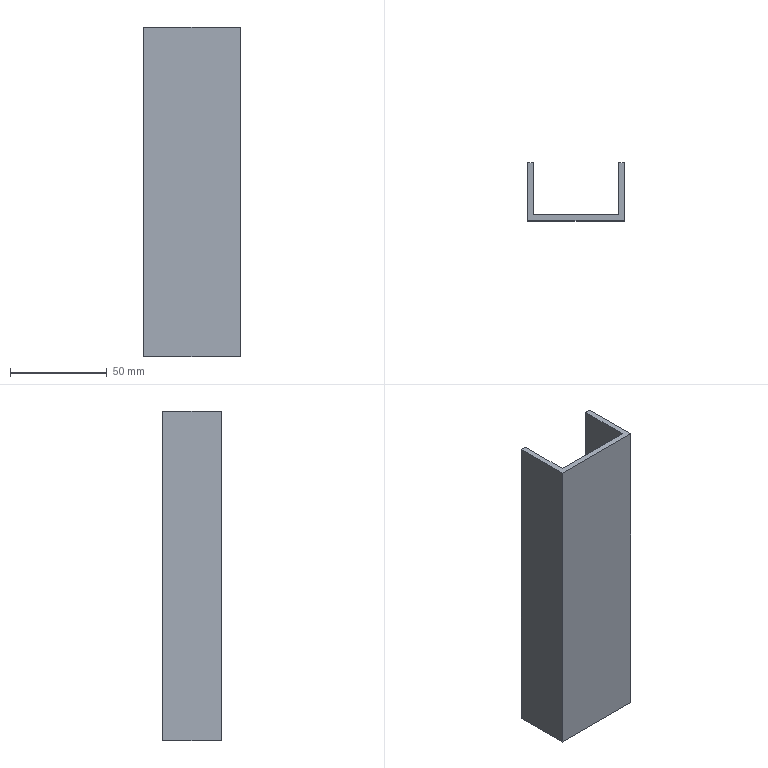Part | SolidWorks | features Extrusion 1, ICE 1 | 1 solid | 10 faces | box 50 x 30 x 170 mm | volume 53040 mm3 | plane 10
STEP:
#1=CARTESIAN_POINT('',(0.,0.,170.));
#2=VERTEX_POINT('',#1);
#3=CARTESIAN_POINT('',(50.,0.,170.));
#4=VERTEX_POINT('',#3);
#5=CARTESIAN_POINT('',(0.,0.,170.));
#6=DIRECTION('',(1.,0.,0.));
#7=VECTOR('',#6,1000.);
#8=LINE('',#5,#7);
#9=EDGE_CURVE('',#2,#4,#8,.T.);
#10=ORIENTED_EDGE('',*,*,#9,.F.);
#11=CARTESIAN_POINT('',(0.,0.,0.));
#12=VERTEX_POINT('',#11);
#13=CARTESIAN_POINT('',(0.,0.,340.));
#14=DIRECTION('',(0.,0.,-1.));
#15=VECTOR('',#14,1000.);
#16=LINE('',#13,#15);
#17=EDGE_CURVE('',#2,#12,#16,.T.);
#18=ORIENTED_EDGE('',*,*,#17,.T.);
#19=CARTESIAN_POINT('',(50.,0.,0.));
#20=VERTEX_POINT('',#19);
#21=CARTESIAN_POINT('',(0.,0.,0.));
#22=DIRECTION('',(1.,0.,0.));
#23=VECTOR('',#22,1000.);
#24=LINE('',#21,#23);
#25=EDGE_CURVE('',#12,#20,#24,.T.);
#26=ORIENTED_EDGE('',*,*,#25,.T.);
#27=CARTESIAN_POINT('',(50.,0.,340.));
#28=DIRECTION('',(0.,0.,-1.));
#29=VECTOR('',#28,1000.);
#30=LINE('',#27,#29);
#31=EDGE_CURVE('',#4,#20,#30,.T.);
#32=ORIENTED_EDGE('',*,*,#31,.F.);
#33=EDGE_LOOP('',(#10,#18,#26,#32));
#34=FACE_OUTER_BOUND('',#33,.T.);
#35=CARTESIAN_POINT('',(0.,0.,340.));
#36=DIRECTION('',(0.,1.,0.));
#37=DIRECTION('',(0.,0.,1.));
#38=AXIS2_PLACEMENT_3D('',#35,#36,#37);
#39=PLANE('',#38);
#40=ADVANCED_FACE('',(#34),#39,.F.);
#41=CARTESIAN_POINT('',(50.,30.,170.));
#42=VERTEX_POINT('',#41);
#43=CARTESIAN_POINT('',(50.,0.,170.));
#44=DIRECTION('',(0.,1.,0.));
#45=VECTOR('',#44,1000.);
#46=LINE('',#43,#45);
#47=EDGE_CURVE('',#4,#42,#46,.T.);
#48=ORIENTED_EDGE('',*,*,#47,.F.);
#49=ORIENTED_EDGE('',*,*,#31,.T.);
#50=CARTESIAN_POINT('',(50.,30.,0.));
#51=VERTEX_POINT('',#50);
#52=CARTESIAN_POINT('',(50.,0.,0.));
#53=DIRECTION('',(0.,1.,0.));
#54=VECTOR('',#53,1000.);
#55=LINE('',#52,#54);
#56=EDGE_CURVE('',#20,#51,#55,.T.);
#57=ORIENTED_EDGE('',*,*,#56,.T.);
#58=CARTESIAN_POINT('',(50.,30.,340.));
#59=DIRECTION('',(0.,0.,-1.));
#60=VECTOR('',#59,1000.);
#61=LINE('',#58,#60);
#62=EDGE_CURVE('',#42,#51,#61,.T.);
#63=ORIENTED_EDGE('',*,*,#62,.F.);
#64=EDGE_LOOP('',(#48,#49,#57,#63));
#65=FACE_OUTER_BOUND('',#64,.T.);
#66=CARTESIAN_POINT('',(50.,0.,340.));
#67=DIRECTION('',(-1.,0.,0.));
#68=DIRECTION('',(0.,0.,1.));
#69=AXIS2_PLACEMENT_3D('',#66,#67,#68);
#70=PLANE('',#69);
#71=ADVANCED_FACE('',(#65),#70,.F.);
#72=CARTESIAN_POINT('',(47.,30.,170.));
#73=VERTEX_POINT('',#72);
#74=CARTESIAN_POINT('',(50.,30.,170.));
#75=DIRECTION('',(-1.,0.,0.));
#76=VECTOR('',#75,1000.);
#77=LINE('',#74,#76);
#78=EDGE_CURVE('',#42,#73,#77,.T.);
#79=ORIENTED_EDGE('',*,*,#78,.F.);
#80=ORIENTED_EDGE('',*,*,#62,.T.);
#81=CARTESIAN_POINT('',(47.,30.,0.));
#82=VERTEX_POINT('',#81);
#83=CARTESIAN_POINT('',(47.,30.,0.));
#84=DIRECTION('',(-1.,0.,0.));
#85=VECTOR('',#84,1000.);
#86=LINE('',#83,#85);
#87=EDGE_CURVE('',#51,#82,#86,.T.);
#88=ORIENTED_EDGE('',*,*,#87,.T.);
#89=CARTESIAN_POINT('',(47.,30.,340.));
#90=DIRECTION('',(0.,0.,-1.));
#91=VECTOR('',#90,1000.);
#92=LINE('',#89,#91);
#93=EDGE_CURVE('',#73,#82,#92,.T.);
#94=ORIENTED_EDGE('',*,*,#93,.F.);
#95=EDGE_LOOP('',(#79,#80,#88,#94));
#96=FACE_OUTER_BOUND('',#95,.T.);
#97=CARTESIAN_POINT('',(47.,30.,340.));
#98=DIRECTION('',(0.,-1.,0.));
#99=DIRECTION('',(0.,0.,-1.));
#100=AXIS2_PLACEMENT_3D('',#97,#98,#99);
#101=PLANE('',#100);
#102=ADVANCED_FACE('',(#96),#101,.F.);
#103=CARTESIAN_POINT('',(47.,3.,170.));
#104=VERTEX_POINT('',#103);
#105=CARTESIAN_POINT('',(47.,30.,170.));
#106=DIRECTION('',(0.,-1.,0.));
#107=VECTOR('',#106,1000.);
#108=LINE('',#105,#107);
#109=EDGE_CURVE('',#73,#104,#108,.T.);
#110=ORIENTED_EDGE('',*,*,#109,.F.);
#111=ORIENTED_EDGE('',*,*,#93,.T.);
#112=CARTESIAN_POINT('',(47.,3.,0.));
#113=VERTEX_POINT('',#112);
#114=CARTESIAN_POINT('',(47.,3.,0.));
#115=DIRECTION('',(0.,-1.,0.));
#116=VECTOR('',#115,1000.);
#117=LINE('',#114,#116);
#118=EDGE_CURVE('',#82,#113,#117,.T.);
#119=ORIENTED_EDGE('',*,*,#118,.T.);
#120=CARTESIAN_POINT('',(47.,3.,340.));
#121=DIRECTION('',(0.,0.,-1.));
#122=VECTOR('',#121,1000.);
#123=LINE('',#120,#122);
#124=EDGE_CURVE('',#104,#113,#123,.T.);
#125=ORIENTED_EDGE('',*,*,#124,.F.);
#126=EDGE_LOOP('',(#110,#111,#119,#125));
#127=FACE_OUTER_BOUND('',#126,.T.);
#128=CARTESIAN_POINT('',(47.,3.,340.));
#129=DIRECTION('',(1.,0.,0.));
#130=DIRECTION('',(0.,0.,-1.));
#131=AXIS2_PLACEMENT_3D('',#128,#129,#130);
#132=PLANE('',#131);
#133=ADVANCED_FACE('',(#127),#132,.F.);
#134=CARTESIAN_POINT('',(3.,3.,170.));
#135=VERTEX_POINT('',#134);
#136=CARTESIAN_POINT('',(47.,3.,170.));
#137=DIRECTION('',(-1.,0.,0.));
#138=VECTOR('',#137,1000.);
#139=LINE('',#136,#138);
#140=EDGE_CURVE('',#104,#135,#139,.T.);
#141=ORIENTED_EDGE('',*,*,#140,.F.);
#142=ORIENTED_EDGE('',*,*,#124,.T.);
#143=CARTESIAN_POINT('',(3.,3.,0.));
#144=VERTEX_POINT('',#143);
#145=CARTESIAN_POINT('',(3.,3.,0.));
#146=DIRECTION('',(-1.,0.,0.));
#147=VECTOR('',#146,1000.);
#148=LINE('',#145,#147);
#149=EDGE_CURVE('',#113,#144,#148,.T.);
#150=ORIENTED_EDGE('',*,*,#149,.T.);
#151=CARTESIAN_POINT('',(3.,3.,340.));
#152=DIRECTION('',(0.,0.,-1.));
#153=VECTOR('',#152,1000.);
#154=LINE('',#151,#153);
#155=EDGE_CURVE('',#135,#144,#154,.T.);
#156=ORIENTED_EDGE('',*,*,#155,.F.);
#157=EDGE_LOOP('',(#141,#142,#150,#156));
#158=FACE_OUTER_BOUND('',#157,.T.);
#159=CARTESIAN_POINT('',(3.,3.,340.));
#160=DIRECTION('',(0.,-1.,0.));
#161=DIRECTION('',(0.,0.,-1.));
#162=AXIS2_PLACEMENT_3D('',#159,#160,#161);
#163=PLANE('',#162);
#164=ADVANCED_FACE('',(#158),#163,.F.);
#165=CARTESIAN_POINT('',(3.,30.,170.));
#166=VERTEX_POINT('',#165);
#167=CARTESIAN_POINT('',(3.,3.,170.));
#168=DIRECTION('',(0.,1.,0.));
#169=VECTOR('',#168,1000.);
#170=LINE('',#167,#169);
#171=EDGE_CURVE('',#135,#166,#170,.T.);
#172=ORIENTED_EDGE('',*,*,#171,.F.);
#173=ORIENTED_EDGE('',*,*,#155,.T.);
#174=CARTESIAN_POINT('',(3.,30.,0.));
#175=VERTEX_POINT('',#174);
#176=CARTESIAN_POINT('',(3.,3.,0.));
#177=DIRECTION('',(0.,1.,0.));
#178=VECTOR('',#177,1000.);
#179=LINE('',#176,#178);
#180=EDGE_CURVE('',#144,#175,#179,.T.);
#181=ORIENTED_EDGE('',*,*,#180,.T.);
#182=CARTESIAN_POINT('',(3.,30.,340.));
#183=DIRECTION('',(0.,0.,-1.));
#184=VECTOR('',#183,1000.);
#185=LINE('',#182,#184);
#186=EDGE_CURVE('',#166,#175,#185,.T.);
#187=ORIENTED_EDGE('',*,*,#186,.F.);
#188=EDGE_LOOP('',(#172,#173,#181,#187));
#189=FACE_OUTER_BOUND('',#188,.T.);
#190=CARTESIAN_POINT('',(3.,3.,340.));
#191=DIRECTION('',(-1.,0.,0.));
#192=DIRECTION('',(0.,0.,1.));
#193=AXIS2_PLACEMENT_3D('',#190,#191,#192);
#194=PLANE('',#193);
#195=ADVANCED_FACE('',(#189),#194,.F.);
#196=CARTESIAN_POINT('',(0.,30.,170.));
#197=VERTEX_POINT('',#196);
#198=CARTESIAN_POINT('',(3.,30.,170.));
#199=DIRECTION('',(-1.,0.,0.));
#200=VECTOR('',#199,1000.);
#201=LINE('',#198,#200);
#202=EDGE_CURVE('',#166,#197,#201,.T.);
#203=ORIENTED_EDGE('',*,*,#202,.F.);
#204=ORIENTED_EDGE('',*,*,#186,.T.);
#205=CARTESIAN_POINT('',(0.,30.,0.));
#206=VERTEX_POINT('',#205);
#207=CARTESIAN_POINT('',(0.,30.,0.));
#208=DIRECTION('',(-1.,0.,0.));
#209=VECTOR('',#208,1000.);
#210=LINE('',#207,#209);
#211=EDGE_CURVE('',#175,#206,#210,.T.);
#212=ORIENTED_EDGE('',*,*,#211,.T.);
#213=CARTESIAN_POINT('',(0.,30.,340.));
#214=DIRECTION('',(0.,0.,-1.));
#215=VECTOR('',#214,1000.);
#216=LINE('',#213,#215);
#217=EDGE_CURVE('',#197,#206,#216,.T.);
#218=ORIENTED_EDGE('',*,*,#217,.F.);
#219=EDGE_LOOP('',(#203,#204,#212,#218));
#220=FACE_OUTER_BOUND('',#219,.T.);
#221=CARTESIAN_POINT('',(0.,30.,340.));
#222=DIRECTION('',(0.,-1.,0.));
#223=DIRECTION('',(0.,0.,-1.));
#224=AXIS2_PLACEMENT_3D('',#221,#222,#223);
#225=PLANE('',#224);
#226=ADVANCED_FACE('',(#220),#225,.F.);
#227=CARTESIAN_POINT('',(0.,30.,170.));
#228=DIRECTION('',(0.,-1.,0.));
#229=VECTOR('',#228,1000.);
#230=LINE('',#227,#229);
#231=EDGE_CURVE('',#197,#2,#230,.T.);
#232=ORIENTED_EDGE('',*,*,#231,.F.);
#233=ORIENTED_EDGE('',*,*,#217,.T.);
#234=CARTESIAN_POINT('',(0.,0.,0.));
#235=DIRECTION('',(0.,-1.,0.));
#236=VECTOR('',#235,1000.);
#237=LINE('',#234,#236);
#238=EDGE_CURVE('',#206,#12,#237,.T.);
#239=ORIENTED_EDGE('',*,*,#238,.T.);
#240=ORIENTED_EDGE('',*,*,#17,.F.);
#241=EDGE_LOOP('',(#232,#233,#239,#240));
#242=FACE_OUTER_BOUND('',#241,.T.);
#243=CARTESIAN_POINT('',(0.,0.,340.));
#244=DIRECTION('',(1.,0.,0.));
#245=DIRECTION('',(0.,0.,-1.));
#246=AXIS2_PLACEMENT_3D('',#243,#244,#245);
#247=PLANE('',#246);
#248=ADVANCED_FACE('',(#242),#247,.F.);
#249=ORIENTED_EDGE('',*,*,#25,.F.);
#250=ORIENTED_EDGE('',*,*,#238,.F.);
#251=ORIENTED_EDGE('',*,*,#211,.F.);
#252=ORIENTED_EDGE('',*,*,#180,.F.);
#253=ORIENTED_EDGE('',*,*,#149,.F.);
#254=ORIENTED_EDGE('',*,*,#118,.F.);
#255=ORIENTED_EDGE('',*,*,#87,.F.);
#256=ORIENTED_EDGE('',*,*,#56,.F.);
#257=EDGE_LOOP('',(#249,#250,#251,#252,#253,#254,#255,#256));
#258=FACE_OUTER_BOUND('',#257,.T.);
#259=CARTESIAN_POINT('',(0.,0.,0.));
#260=DIRECTION('',(0.,0.,1.));
#261=DIRECTION('',(1.,0.,0.));
#262=AXIS2_PLACEMENT_3D('',#259,#260,#261);
#263=PLANE('',#262);
#264=ADVANCED_FACE('',(#258),#263,.F.);
#265=ORIENTED_EDGE('',*,*,#231,.T.);
#266=ORIENTED_EDGE('',*,*,#9,.T.);
#267=ORIENTED_EDGE('',*,*,#47,.T.);
#268=ORIENTED_EDGE('',*,*,#78,.T.);
#269=ORIENTED_EDGE('',*,*,#109,.T.);
#270=ORIENTED_EDGE('',*,*,#140,.T.);
#271=ORIENTED_EDGE('',*,*,#171,.T.);
#272=ORIENTED_EDGE('',*,*,#202,.T.);
#273=EDGE_LOOP('',(#265,#266,#267,#268,#269,#270,#271,#272));
#274=FACE_OUTER_BOUND('',#273,.T.);
#275=CARTESIAN_POINT('',(0.,0.,170.));
#276=DIRECTION('',(0.,0.,1.));
#277=DIRECTION('',(1.,0.,0.));
#278=AXIS2_PLACEMENT_3D('',#275,#276,#277);
#279=PLANE('',#278);
#280=ADVANCED_FACE('',(#274),#279,.T.);
#281=CLOSED_SHELL('',(#40,#71,#102,#133,#164,#195,#226,#248,#264,#280));
#282=MANIFOLD_SOLID_BREP('',#281);
#283=CARTESIAN_POINT('',(0.,0.,0.));
#284=DIRECTION('',(0.,0.,1.));
#285=DIRECTION('',(1.,0.,0.));
#286=AXIS2_PLACEMENT_3D('',#283,#284,#285);
#287=(LENGTH_UNIT()NAMED_UNIT(*)SI_UNIT(.MILLI.,.METRE.));
#288=UNCERTAINTY_MEASURE_WITH_UNIT(LENGTH_MEASURE(0.00001),#287,'','');
#289=(NAMED_UNIT(*)PLANE_ANGLE_UNIT()SI_UNIT($,.RADIAN.));
#290=(NAMED_UNIT(*)SI_UNIT($,.STERADIAN.)SOLID_ANGLE_UNIT());
#291=(GEOMETRIC_REPRESENTATION_CONTEXT(3)GLOBAL_UNCERTAINTY_ASSIGNED_CONTEXT((#288))GLOBAL_UNIT_ASSIGNED_CONTEXT((#287,#289,#290))REPRESENTATION_CONTEXT('',''));
#292=ADVANCED_BREP_SHAPE_REPRESENTATION('',(#282,#286),#291);